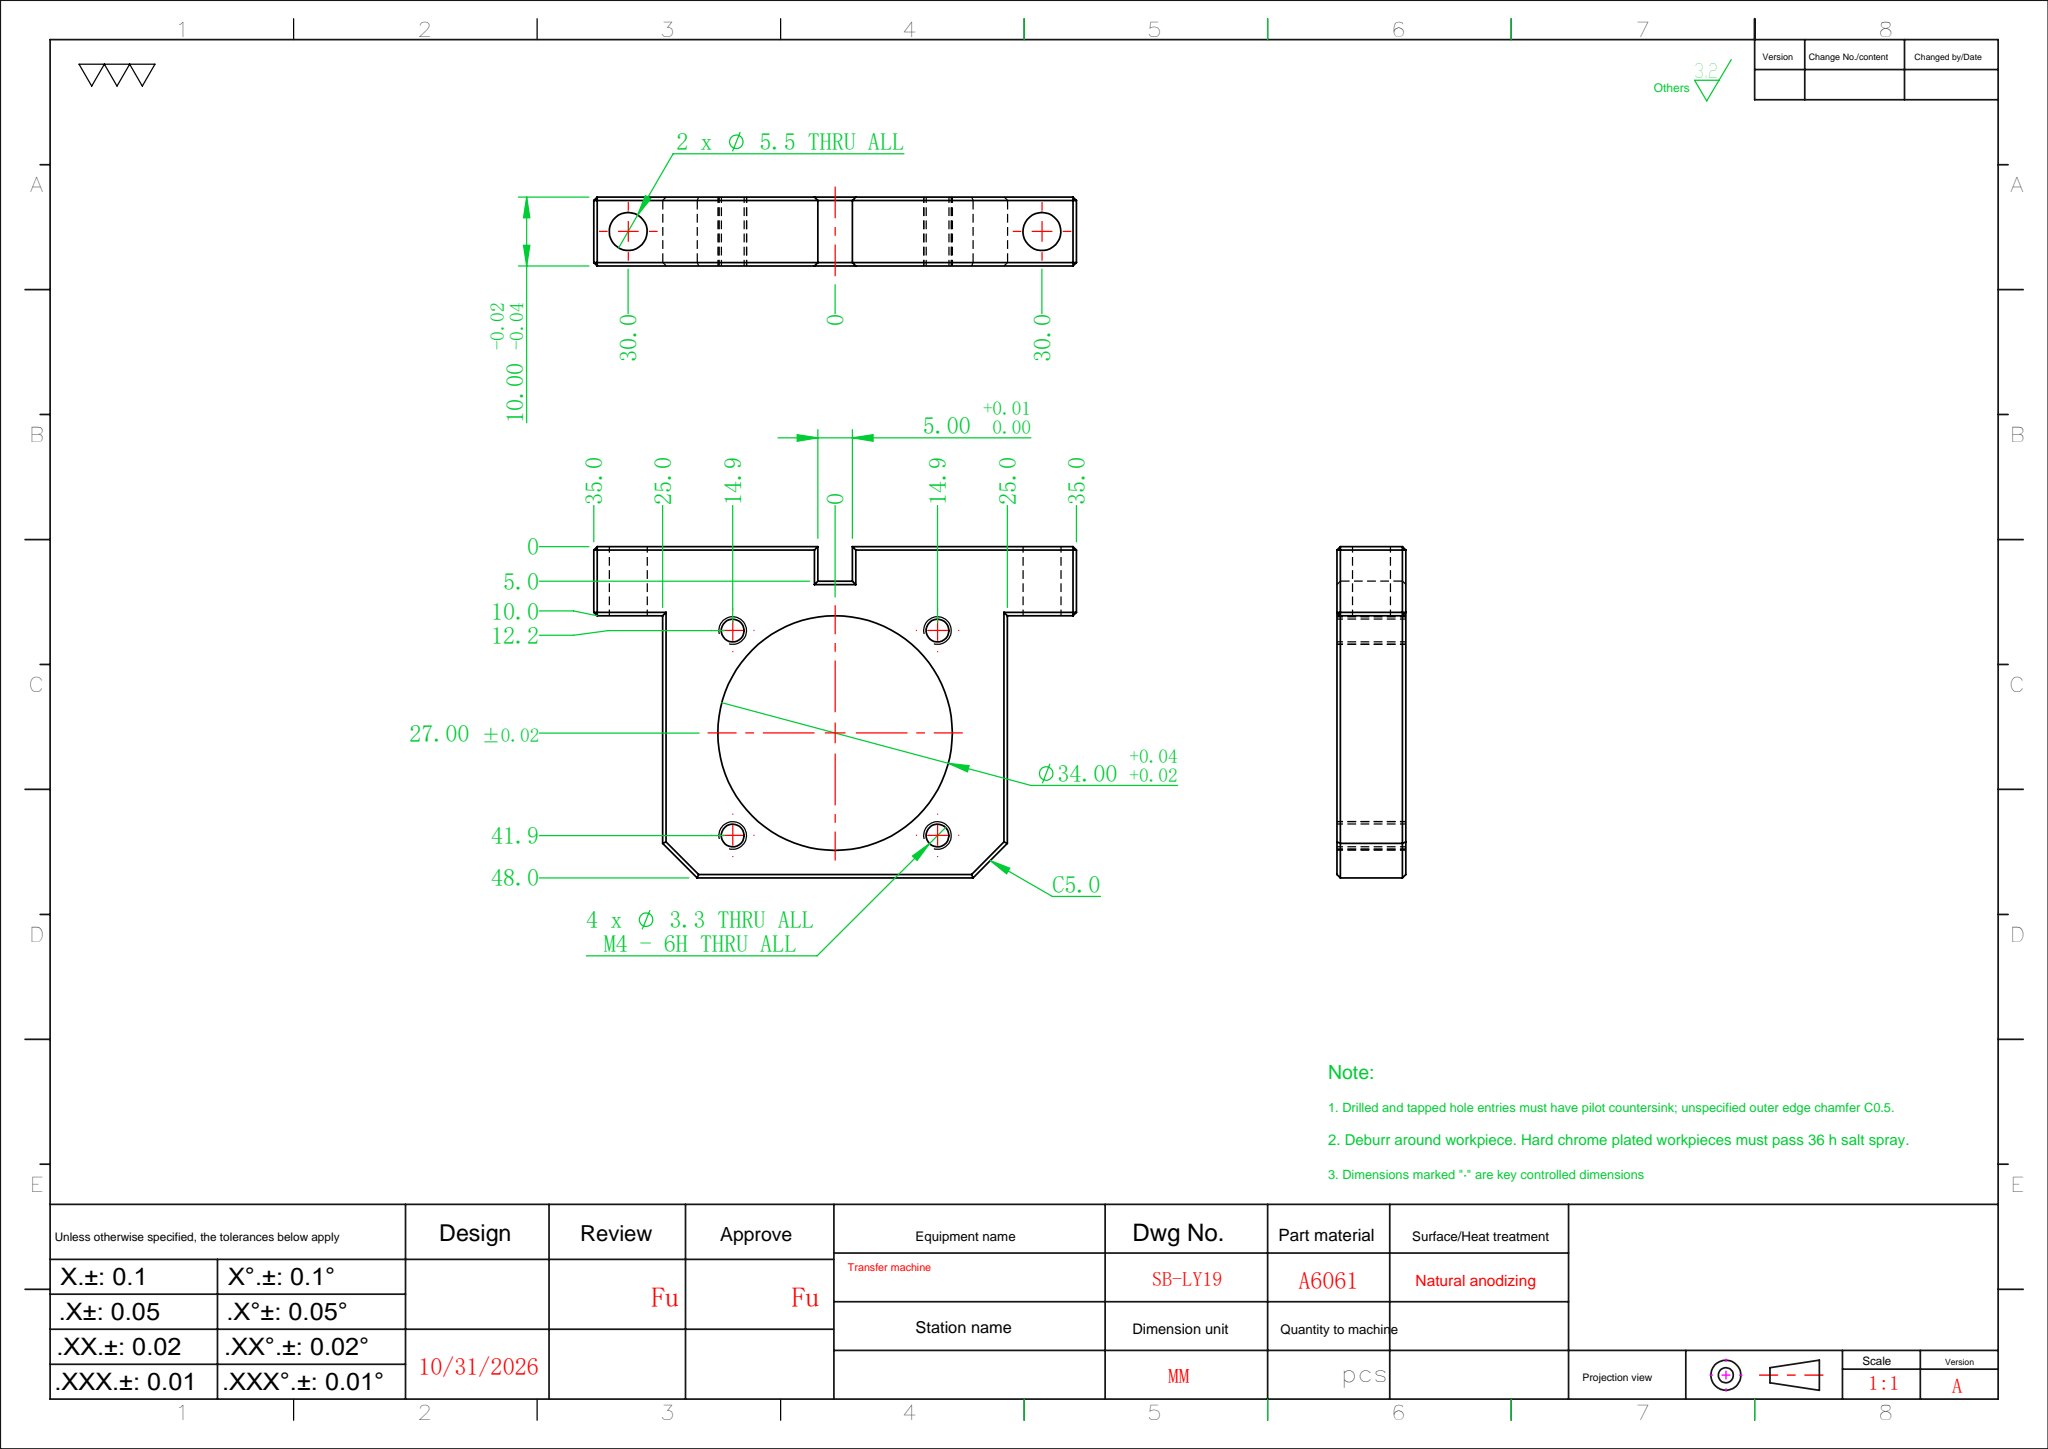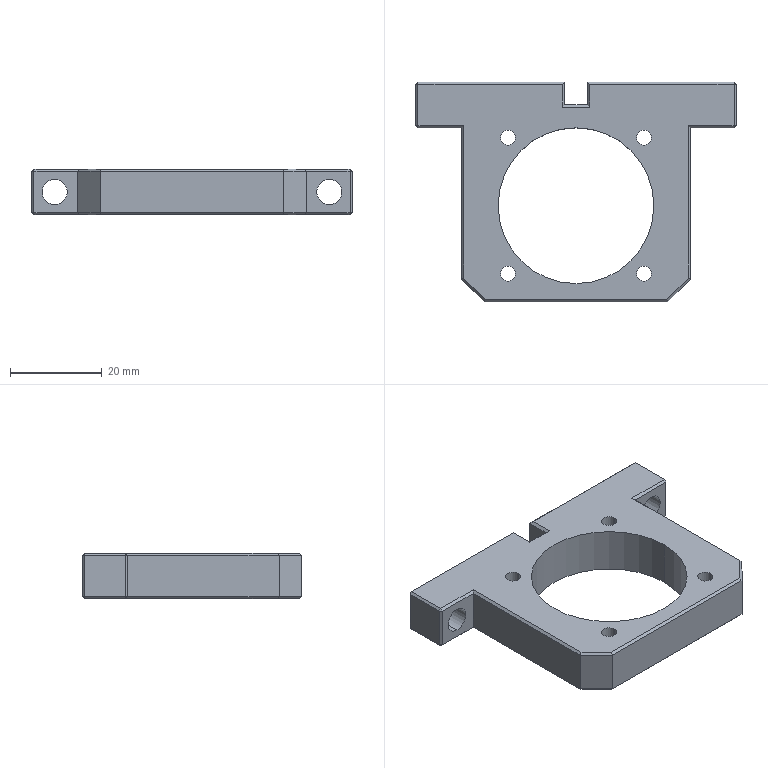Part | SolidWorks | features Chamfer 2, Cut 2, HoleWzd 2, Extrusion 1, ICE 1 | 1 solid | 70 faces | box 70 x 48 x 10 mm | volume 15539 mm3 | plane 56 | cylinder 14 | commonest cylinder face diameters 3.3 x8 5.5 x4 34 x2